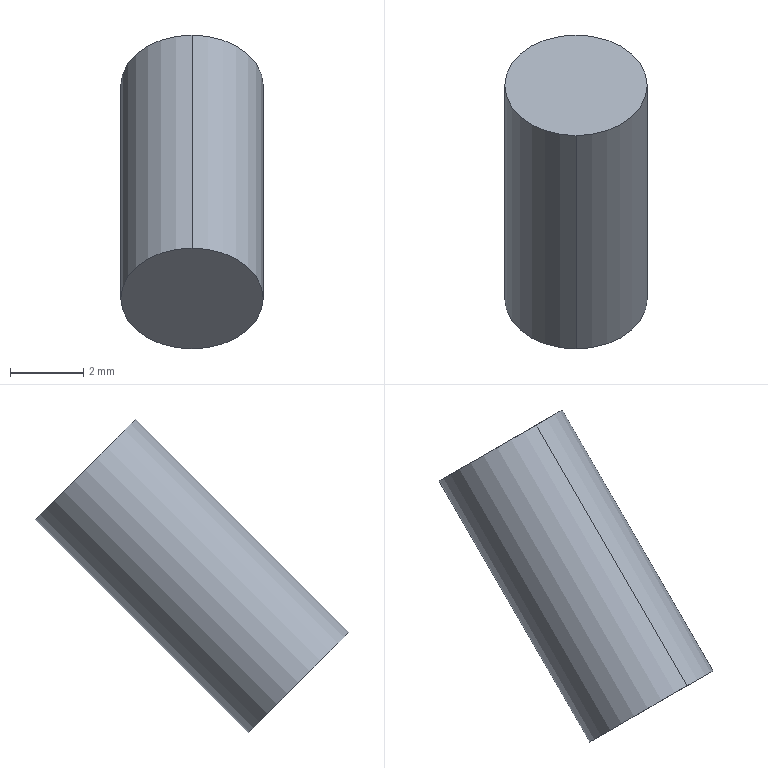Part | STEP file | PZ-G51EP-Part-2-11 | 1 solid | 4 faces | box 3.9 x 8.588 x 8.588 mm | volume 98.5 mm3 | cylinder 2 | plane 2 | commonest cylinder face diameters 3.9 x2
STEP:
#1=CARTESIAN_POINT('',(0.,-21.32,-33.012));
#2=VERTEX_POINT('',#1);
#3=CARTESIAN_POINT('',(0.,-18.562,-35.77));
#4=VERTEX_POINT('',#3);
#5=CARTESIAN_POINT('',(0.,-19.941,-34.391));
#6=DIRECTION('',(0.,0.7071,0.7071));
#7=DIRECTION('',(0.,-0.7071,0.7071));
#8=AXIS2_PLACEMENT_3D('',#5,#6,#7);
#9=CIRCLE('',#8,1.95);
#10=EDGE_CURVE('',#2,#4,#9,.T.);
#11=ORIENTED_EDGE('',*,*,#10,.T.);
#12=CARTESIAN_POINT('',(0.,-12.732,-29.94));
#13=VERTEX_POINT('',#12);
#14=CARTESIAN_POINT('',(0.,-11.491,-28.699));
#15=DIRECTION('',(0.,0.7071,0.7071));
#16=VECTOR('',#15,1000.);
#17=LINE('',#14,#16);
#18=EDGE_CURVE('',#4,#13,#17,.T.);
#19=ORIENTED_EDGE('',*,*,#18,.T.);
#20=CARTESIAN_POINT('',(0.,-15.49,-27.182));
#21=VERTEX_POINT('',#20);
#22=CARTESIAN_POINT('',(0.,-14.111,-28.561));
#23=DIRECTION('',(0.,0.7071,0.7071));
#24=DIRECTION('',(0.,-0.7071,0.7071));
#25=AXIS2_PLACEMENT_3D('',#22,#23,#24);
#26=CIRCLE('',#25,1.95);
#27=EDGE_CURVE('',#21,#13,#26,.T.);
#28=ORIENTED_EDGE('',*,*,#27,.F.);
#29=CARTESIAN_POINT('',(0.,-14.249,-25.941));
#30=DIRECTION('',(0.,0.7071,0.7071));
#31=VECTOR('',#30,1000.);
#32=LINE('',#29,#31);
#33=EDGE_CURVE('',#2,#21,#32,.T.);
#34=ORIENTED_EDGE('',*,*,#33,.F.);
#35=EDGE_LOOP('',(#11,#19,#28,#34));
#36=FACE_OUTER_BOUND('',#35,.T.);
#37=CARTESIAN_POINT('',(0.,-12.87,-27.32));
#38=DIRECTION('',(0.,0.7071,0.7071));
#39=DIRECTION('',(0.,-0.7071,0.7071));
#40=AXIS2_PLACEMENT_3D('',#37,#38,#39);
#41=CYLINDRICAL_SURFACE('',#40,1.95);
#42=ADVANCED_FACE('',(#36),#41,.T.);
#43=ORIENTED_EDGE('',*,*,#18,.F.);
#44=CARTESIAN_POINT('',(0.,-19.941,-34.391));
#45=DIRECTION('',(0.,0.7071,0.7071));
#46=DIRECTION('',(0.,-0.7071,0.7071));
#47=AXIS2_PLACEMENT_3D('',#44,#45,#46);
#48=CIRCLE('',#47,1.95);
#49=EDGE_CURVE('',#4,#2,#48,.T.);
#50=ORIENTED_EDGE('',*,*,#49,.T.);
#51=ORIENTED_EDGE('',*,*,#33,.T.);
#52=CARTESIAN_POINT('',(0.,-14.111,-28.561));
#53=DIRECTION('',(0.,0.7071,0.7071));
#54=DIRECTION('',(0.,-0.7071,0.7071));
#55=AXIS2_PLACEMENT_3D('',#52,#53,#54);
#56=CIRCLE('',#55,1.95);
#57=EDGE_CURVE('',#13,#21,#56,.T.);
#58=ORIENTED_EDGE('',*,*,#57,.F.);
#59=EDGE_LOOP('',(#43,#50,#51,#58));
#60=FACE_OUTER_BOUND('',#59,.T.);
#61=CARTESIAN_POINT('',(0.,-12.87,-27.32));
#62=DIRECTION('',(0.,0.7071,0.7071));
#63=DIRECTION('',(0.,-0.7071,0.7071));
#64=AXIS2_PLACEMENT_3D('',#61,#62,#63);
#65=CYLINDRICAL_SURFACE('',#64,1.95);
#66=ADVANCED_FACE('',(#60),#65,.T.);
#67=ORIENTED_EDGE('',*,*,#10,.F.);
#68=ORIENTED_EDGE('',*,*,#49,.F.);
#69=EDGE_LOOP('',(#67,#68));
#70=FACE_OUTER_BOUND('',#69,.T.);
#71=CARTESIAN_POINT('',(0.,-18.562,-35.77));
#72=DIRECTION('',(0.,0.7071,0.7071));
#73=DIRECTION('',(0.,-0.7071,0.7071));
#74=AXIS2_PLACEMENT_3D('',#71,#72,#73);
#75=PLANE('',#74);
#76=ADVANCED_FACE('',(#70),#75,.F.);
#77=ORIENTED_EDGE('',*,*,#27,.T.);
#78=ORIENTED_EDGE('',*,*,#57,.T.);
#79=EDGE_LOOP('',(#77,#78));
#80=FACE_OUTER_BOUND('',#79,.T.);
#81=CARTESIAN_POINT('',(0.,-12.732,-29.94));
#82=DIRECTION('',(0.,-0.7071,-0.7071));
#83=DIRECTION('',(0.,0.7071,-0.7071));
#84=AXIS2_PLACEMENT_3D('',#81,#82,#83);
#85=PLANE('',#84);
#86=ADVANCED_FACE('',(#80),#85,.F.);
#87=CLOSED_SHELL('',(#42,#66,#76,#86));
#88=MANIFOLD_SOLID_BREP('',#87);
#89=CARTESIAN_POINT('',(0.,0.,0.));
#90=DIRECTION('',(0.,0.,1.));
#91=DIRECTION('',(1.,0.,0.));
#92=AXIS2_PLACEMENT_3D('',#89,#90,#91);
#93=(LENGTH_UNIT()NAMED_UNIT(*)SI_UNIT(.MILLI.,.METRE.));
#94=UNCERTAINTY_MEASURE_WITH_UNIT(LENGTH_MEASURE(0.00001),#93,'','');
#95=(NAMED_UNIT(*)PLANE_ANGLE_UNIT()SI_UNIT($,.RADIAN.));
#96=(NAMED_UNIT(*)SI_UNIT($,.STERADIAN.)SOLID_ANGLE_UNIT());
#97=(GEOMETRIC_REPRESENTATION_CONTEXT(3)GLOBAL_UNCERTAINTY_ASSIGNED_CONTEXT((#94))GLOBAL_UNIT_ASSIGNED_CONTEXT((#93,#95,#96))REPRESENTATION_CONTEXT('',''));
#98=ADVANCED_BREP_SHAPE_REPRESENTATION('',(#88,#92),#97);